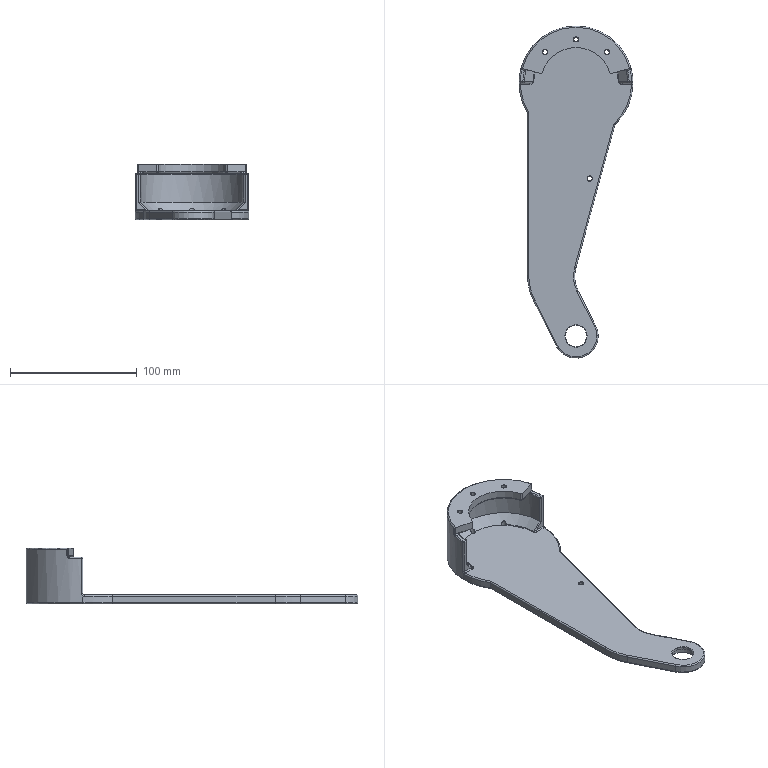Part | SolidWorks | features ICE 8, Fillet 4, Chamfer 1, Extrusion 1 | 1 solid | 153 faces | box 90 x 262.5 x 44 mm | volume 128992 mm3 | cylinder 62 | torus 54 | plane 19 | spline 10 | sphere 7 | cone 1 | commonest cylinder face diameters 2 x28 3.7 x14 6 x8 90 x4 17 x2 21.15 x2